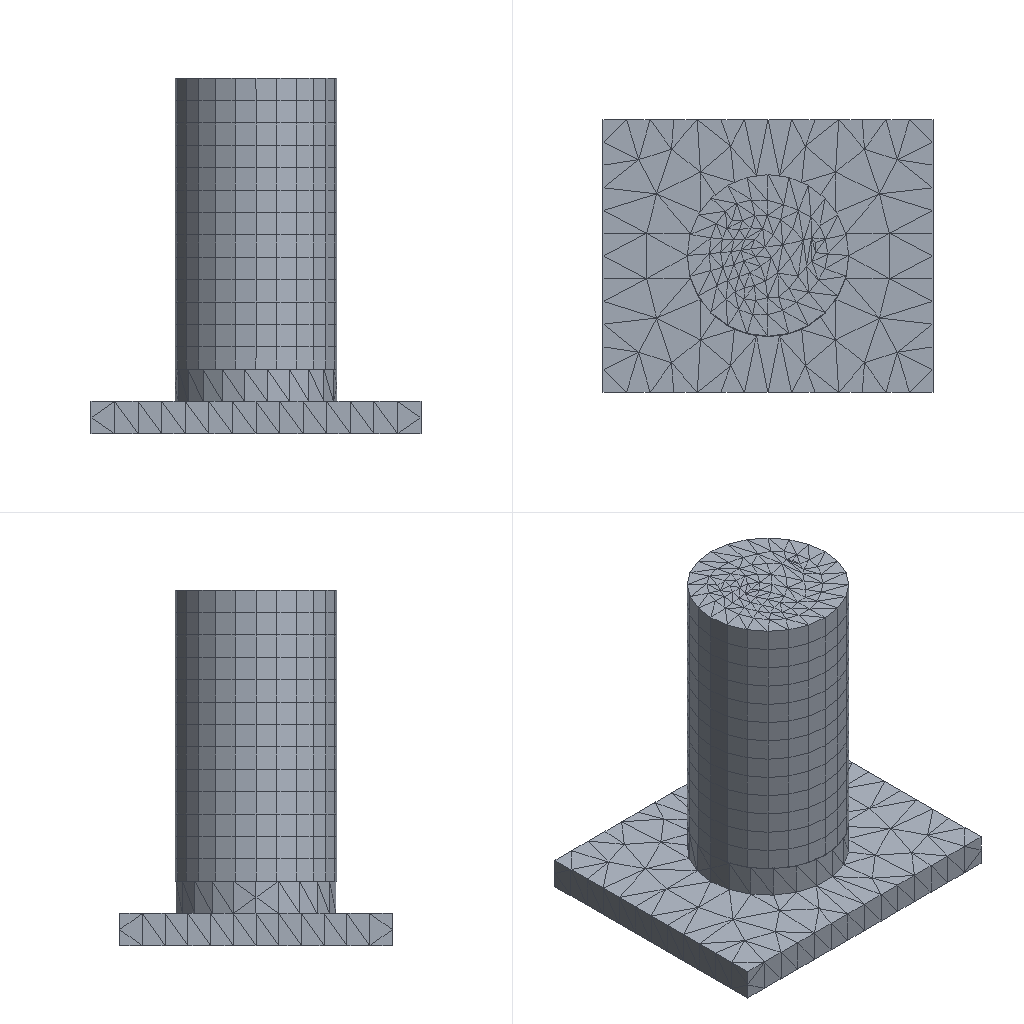Simulation study | ansys workbench
Set-up summary:
category,name,step,type,value,unit,region
solver,ansys_workbench
units,mm-N-s-tonne (MPa),,stated,"/units,MPA"
analysis,LS1,,static
load_step,LS1,LS1,static,nsubst=1; time=1
mesh,nodes,,,6476
mesh,elements,,,2149
element_type,SOLID186,,,1092
element_type,SOLID187,,,649
element_type,CONTA174,,,288
element_type,TARGE170,,,120
material,Structural Steel,,E,200000,tonne s^-2 mm^-1
material,Structural Steel,,nu,0.3
material,Structural Steel,,density,7.85e-09,tonne mm^-3
material,Structural Steel,,conductivity,60.5,tonne mm s^-3 C^-1
material,Structural Steel,,specific_heat,4.34e+08,mm^2 s^-2 C^-1
material,Structural Steel,,cte,1.2e-05,C^-1
material,Structural Steel,,permeability,10000
material,Structural Steel,,resistivity,0.00017,ohm mm
load,,LS1,force,"5381.45 [dir=(-0.7433, -0.669, 0) n=6]",,all
bc,Fixed Supports,model,fixed,[dofs=ALL],,_FIXEDSU
contact,Contact Region,,bonded (always),element=CONTA174
contact,contact 2,,bonded (always),element=CONTA174
contact,contact 3,,bonded (always),element=CONTA174
named_set,_FIXEDSU,,node,321
Ansys APDL input file, long lists of numbers shortened:
/batch
/config,noeldb,1     ! force off writing results to database
*get,_wallstrt,active,,time,wall
! ANSYS input file written by Workbench version 2021 R1
! File used for geometry attach:
/title,wbnew--____ (B5)
! ****** Begin Custom Load Command Snippet ******
/COM, ACT Extensions:
/COM,     LSDYNA, 2021.1
/COM,
! ****** End   Custom Load Command Snippet ******
*DIM,_wb_ProjectScratch_dir,string,248
_wb_ProjectScratch_dir(1) = ''
*DIM,_wb_SolverFiles_dir,string,248
_wb_SolverFiles_dir(1) = ''
*DIM,_wb_userfiles_dir,string,248
_wb_userfiles_dir(1) = ''
/com,--- Data in consistent NMM units. See Solving Units in the help system for more information.
/units,MPA
/nopr
/wb,file,start              !  signify a WB generated input file
/prep7
! Turn off shape checking because checks already performed inside WB mesher.
! See help system for more information.
SHPP,OFF,,NOWARN
/nolist
etcon,set             ! allow ANSYS to choose best KEYOP's for 180x elements, resets any applicable keyopt to MAPDL defaults
/com,*********** Nodes for the whole assembly ***********
nblock,3,,7121
(1i9,3e20.9e3)
        1    -3.919930775E+00    -2.844930224E-01     6.923076923E+00
! (6473 more lines like these left out)
-1
/com,*********** Nodes for all Remote Points ***********
nblock,3
(1i9,3e20.9e3)
     6475    -1.500000000E+02     0.000000000E+00     9.000000000E+01
     6476    -1.500000000E+02     0.000000000E+00     9.000000000E+01
-1
/wb,elem,start            !  set before creation of elements
/com,*********** Elements for Body 1 "__1-FreeParts|__-__1" ***********
et,1,186
keyo,1,2,1          ! set full integration on SOLID186
eblock,19,solid,,1092
(19i9)
        1        1        1        1        0        0        0        0       20        0        1        1       13       49       61      936      935      932      931
! (2183 more lines like these left out)
-1
/com,*********** Elements for Body 2 "__1-FreeParts|__-__3" ***********
et,2,187
eblock,19,solid,,649
(19i9)
        2        2        2        2        0        0        0        0       10        0     1093     5149     5163     5150     5349     5670     5677     5668     5675
! (1297 more lines like these left out)
-1
/wb,elem,end               !  done creating elements
/com,*********** Send User Defined Coordinate System(s) ***********
csys,0
toffst,273.15,  ! Temperature offset from absolute zero
/com,*********** Set Reference Temperature ***********
tref,22.
/wb,mat,start              !  starting to send materials
/com,*********** Send Materials ***********
Temperature = 'TEMP' ! Temperature
MP,DENS,1,7.85e-09,	! tonne mm^-3
MP,ALPX,1,1.2e-05,	! C^-1
MP,C,1,434000000,	! mm^2 s^-2 C^-1
MP,KXX,1,60.5,	! tonne mm s^-3 C^-1
MP,RSVX,1,0.00017,	! ohm mm
MP,EX,1,200000,	! tonne s^-2 mm^-1
MP,NUXY,1,0.3,
MP,MURX,1,10000,
Temperature = 'TEMP' ! Temperature
MP,DENS,2,7.85e-09,	! tonne mm^-3
MP,ALPX,2,1.2e-05,	! C^-1
MP,C,2,434000000,	! mm^2 s^-2 C^-1
MP,KXX,2,60.5,	! tonne mm s^-3 C^-1
MP,RSVX,2,0.00017,	! ohm mm
MP,EX,2,200000,	! tonne s^-2 mm^-1
MP,NUXY,2,0.3,
MP,MURX,2,10000,
/wb,mat,end                !  done sending materials
!************************* Model Summary ********************
!__1-FreeParts|__-__1,	结构钢,	matid,	1
!__1-FreeParts|__-__3,	结构钢,	matid,	2
!************************* End Model Summary ********************
! get the diagonal of the bounding box. Needed later for other things
*get,_xmin,node,,mnloc,x
*get,_ymin,node,,mnloc,y
*get,_zmin,node,,mnloc,z
*get,_xmax,node,,mxloc,x
*get,_ymax,node,,mxloc,y
*get,_zmax,node,,mxloc,z
_ASMDIAG=(_xmax-_xmin)*(_xmax-_xmin)+(_ymax-_ymin)*(_ymax-_ymin)+(_zmax-_zmin)*(_zmax-_zmin)
_ASMDIAG=SQRT(_ASMDIAG)
/wb,contact,start          !  starting to send contact
/com,*********** Create Contact "接触区域" ***********
/com,            Real Constant Set For Above Contact Is 4 & 3
*set,tid,4
*set,cid,3
r,tid
r,cid
et,tid,170
et,cid,174
eblock,10,,,84
(15i9)
     2676        4        4        4        0      911      891      885      885     4238     4217      885     4219
! (83 more lines like these left out)
-1
eblock,10,,,84
(15i9)
     2760        3        3        3        0      911      891      885      885     4238     4217      885     4219
! (83 more lines like these left out)
-1
eblock,10,,,36
(15i9)
     2844        3        4        3        0     5135     5321     5136     5136     5623     5625     5136     5622
! (35 more lines like these left out)
-1
eblock,10,,,36
(15i9)
     2880        4        3        4        0     5135     5321     5136     5136     5623     5625     5136     5622
! (35 more lines like these left out)
-1
keyo,cid,8,2               ! auto create asymmetric contact (from Program Controlled setting)
keyo,cid,10,0              ! adjust contact stiffness each NR iteration (from Program Controlled setting)
keyo,cid,12,5              ! bonded always
keyo,cid,18,1              ! small sliding turned on by application
keyo,cid,2,0               ! augmented Lagrange (from Program Controlled setting)
keyo,cid,4,0               ! on Gauss point (from Program Controlled setting)
keyo,cid,9,1               ! ignore initial gaps/penetration
keyo,cid,7,0               ! No Prediction
rmod,tid,3,10.      ! FKN
rmod,tid,5,0.       ! ICONT
rmod,tid,6,0.       ! PINB
rmod,tid,10,0.      ! CNOF
rmod,tid,12,0.      ! FKT
rmod,tid,36,27      ! WB DSID
rmod,cid,3,10.      ! FKN
rmod,cid,5,0.       ! ICONT
rmod,cid,6,0.       ! PINB
rmod,cid,10,0.      ! CNOF
rmod,cid,12,0.      ! FKT
rmod,cid,36,27      ! WB DSID
nsel,all
esel,all
/wb,contact,end            !  done creating contacts
/golist
/wb,load,start             !  starting to send loads
/com,*********** Fixed Supports ***********
CMBLOCK,_FIXEDSU,NODE,      321
(8i10)
      5158      5160      5161      5162      5163      5164      5165      5166
! (40 more lines like these left out)
cmsel,s,_FIXEDSU
d,all,all
nsel,all
/com,*********** Create Remote Point "内部远程点" ***********
! -------- Remote Point Used by "远程力" --------
*set,tid,6
*set,cid,5
et,cid,174
et,tid,170
keyo,tid,2,1               ! Don't fix the pilot node
keyo,tid,4,111111
keyo,cid,12,5              ! Bonded Contact
keyo,cid,4,1               ! Deformable RBE3 style load
keyo,cid,2,2               ! MPC style contact
eblock,10,,,84
(15i9)
     2916        5        5        5        0      962      988      982      982     4367     4430      982     4365
! (83 more lines like these left out)
-1
*set,_npilot,6475
_npilot38=_npilot
type,tid
mat ,cid
real,cid
tshape,pilo
en,3000,_npilot
tshape
/com,*********** Create Remote Point "内部远程点" ***********
! -------- Remote Point Used by "远程力 2" --------
*set,tid,8
*set,cid,7
et,cid,174
et,tid,170
keyo,tid,2,1               ! Don't fix the pilot node
keyo,tid,4,111111
keyo,cid,12,5              ! Bonded Contact
keyo,cid,4,1               ! Deformable RBE3 style load
keyo,cid,2,2               ! MPC style contact
eblock,10,,,84
(15i9)
     3001        7        7        7        0      962      988      982      982     4367     4430      982     4365
! (83 more lines like these left out)
-1
*set,_npilot,6476
_npilot43=_npilot
type,tid
mat ,cid
real,cid
tshape,pilo
en,3085,_npilot
tshape
/com,*********** Construct Remote Force ***********
/com,*********** Construct Remote Force ***********
/gst,on,on
fini
*get,_numnode,node,0,count
*get,_numelem,elem,0,count
*get, _MAXELEMNUM, elem, 0, NUM, MAX
*get, _MAXNODENUM, node, 0, NUM, MAX
*get, _MAXELEMTYPE, etyp, 0, NUM, MAX
*get, _MAXREALCONST, real, 0, NUM, MAX
/go
/wb,load,end               !  done creating loads
/com,--- Number of total nodes = %_numnode%
/com,--- Number of contact elements = 408
/com,--- Number of spring elements = 0
/com,--- Number of bearing elements = 0
/com,--- Number of solid elements = 1741
/com,--- Number of condensed parts = 0
/com,--- Number of total elements = %_numelem%
*get,_wallbsol,active,,time,wall
/com,****************************************************************************
/com,*************************    SOLUTION       ********************************
/com,****************************************************************************
/solu
antype,0                   ! static analysis
_thickRatio=0.5     ! Ratio of thick parts in the model
eqsl,sparse,,,,,1
cntr,print,1               ! print out contact info and also make no initial contact an error
dmpoption,emat,no             ! Don't combine emat file for DANSYS
dmpoption,esav,no             ! Don't combine esav file for DANSYS
nldiag,cont,iter           ! print out contact info each equilibrium iteration
rescontrol,,none                 ! Do not keep any restart files
/com,****************************************************
/com,******************* SOLVE FOR LS 1 OF 1 ****************
nsel,s,node,,6475
f,all,fx,0.
f,all,fy,-3600.
f,all,fz,0.
nsel,s,node,,6476
f,all,fx,-4000.
f,all,fy,0.
f,all,fz,0.
nsel,all
/nopr
/gopr
/nolist
nsub,1,1,1
time,1.
outres,erase
outres,all,none
outres,nsol,all,
outres,rsol,all
outres,eangl,all
outres,etmp,all
outres,veng,all
outres,strs,all,
outres,epel,all,
outres,eppl,all,
outres,cont,all,
! *********** WB SOLVE COMMAND ***********
! check interactive state
*get,ANSINTER_,active,,int
*if,ANSINTER_,ne,0,then
/eof
*endif
solve
/com *************** Write FE CONNECTORS *********
CEWRITE,file,ce,,INTE
/com,****************************************************
/com,*************** FINISHED SOLVE FOR LS 1 *************
*get,_wallasol,active,,time,wall
/nopr
*get,_numnode,node,0,count
*get,_numelem,elem,0,count
*get, _MAXELEMNUM, elem, 0, NUM, MAX
*get, _MAXNODENUM, node, 0, NUM, MAX,,,INTERNAL
*get, _MAXELEMTYPE, etyp, 0, NUM, MAX
*get, _MAXREALCONST, real, 0, NUM, MAX
/gopr
/post1
xmlo,ENCODING,ISO-8859-1
xmlo,parm
/xml,parm,xml
fini
/gopr
*get,_walldone,active,,time,wall
_preptime=(_wallbsol-_wallstrt)*3600
_solvtime=(_wallasol-_wallbsol)*3600
_posttime=(_walldone-_wallasol)*3600
_totaltim=(_walldone-_wallstrt)*3600
*get,_dlbratio,active,0,solu,dlbr
*get,_combtime,active,0,solu,comb
/com,--- Total number of nodes = %_numnode%
/com,--- Total number of elements = %_numelem%
/com,--- Element load balance ratio = %_dlbratio%
/com,--- Time to combine distributed files = %_combtime%
/wb,file,end               ! done with WB generated input
Results summary:
result,analyses[0].index,,,1
result,analyses[0].system,,,SYS
result,analyses[0].deck,,,deck.dat
result,analyses[0].solve_status,,,completed
result,analyses[0].analysis_type,,,static
result,analyses[0].physics,,,mechanical
result,analyses[0].unit_system,,,"NMM: mm, ton, N, s, mV, mA, degC"
result,analyses[0].n_sets,,,1
result,analyses[0].load_steps[0].set,set=1,,1
result,analyses[0].load_steps[0].time_or_freq,set=1,,1
result,analyses[0].load_steps[0].max_displacement_magnitude,set=1,,0.2144
result,analyses[0].load_steps[0].max_von_mises_nodal,set=1,,57.822
result,analyses[0].load_steps[0].reaction_force_sum_xyz[1],set=1,,4000
result,analyses[0].load_steps[0].reaction_force_sum_xyz[2],set=1,,3600
result,analyses[0].load_steps[0].reaction_force_sum_xyz[3],set=1,,-5.25489e-09